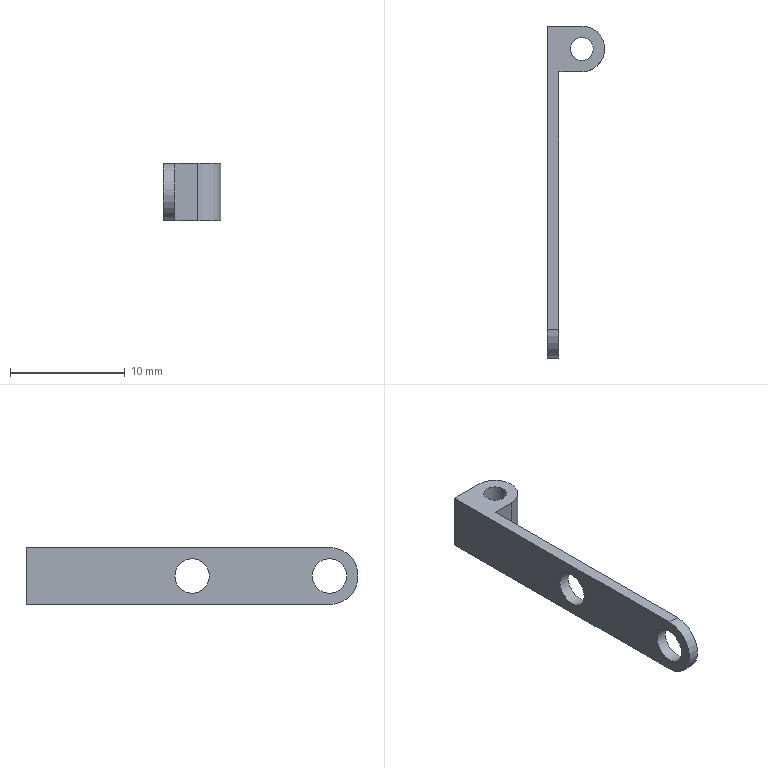Part | STEP file | 1-63.2 | 1 solid | 11 faces | box 5 x 29 x 5 mm | volume 183.888 mm3 | plane 6 | cylinder 5 | commonest cylinder face diameters 3 x2 2 x1 4 x1 5 x1
STEP:
#1=CARTESIAN_POINT('',(0.,0.,0.));
#2=DIRECTION('',(0.,0.,1.));
#3=DIRECTION('',(1.,0.,0.));
#4=AXIS2_PLACEMENT_3D('',#1,#2,#3);
#5=CARTESIAN_POINT('',(0.,0.,2.5));
#6=VERTEX_POINT('',#5);
#7=CARTESIAN_POINT('',(0.,0.,-2.5));
#8=VERTEX_POINT('',#7);
#9=CARTESIAN_POINT('',(0.,0.,0.));
#10=DIRECTION('',(1.,0.,0.));
#11=DIRECTION('',(0.,0.,1.));
#12=AXIS2_PLACEMENT_3D('',#9,#10,#11);
#13=CIRCLE('',#12,2.5);
#14=CARTESIAN_POINT('',(0.,0.,0.));
#15=DIRECTION('',(1.,0.,0.));
#16=DIRECTION('',(0.,0.,1.));
#17=AXIS2_PLACEMENT_3D('',#14,#15,#16);
#18=CYLINDRICAL_SURFACE('',#17,2.5);
#19=CARTESIAN_POINT('',(0.,0.));
#20=DIRECTION('',(1.,0.));
#21=VECTOR('',#20,1.);
#22=LINE('',#19,#21);
#23=(GEOMETRIC_REPRESENTATION_CONTEXT(2)PARAMETRIC_REPRESENTATION_CONTEXT()REPRESENTATION_CONTEXT('',''));
#24=DEFINITIONAL_REPRESENTATION('',(#22),#23);
#25=PCURVE('',#18,#24);
#26=CARTESIAN_POINT('',(0.,14.25,14.25));
#27=DIRECTION('',(1.,0.,0.));
#28=DIRECTION('',(0.,1.,0.));
#29=AXIS2_PLACEMENT_3D('',#26,#27,#28);
#30=PLANE('',#29);
#31=CARTESIAN_POINT('',(-14.25,-14.25));
#32=DIRECTION('',(0.,1.));
#33=AXIS2_PLACEMENT_2D('',#31,#32);
#34=CIRCLE('',#33,2.5);
#35=(GEOMETRIC_REPRESENTATION_CONTEXT(2)PARAMETRIC_REPRESENTATION_CONTEXT()REPRESENTATION_CONTEXT('',''));
#36=DEFINITIONAL_REPRESENTATION('',(#34),#35);
#37=PCURVE('',#30,#36);
#38=SURFACE_CURVE('',#13,(#25,#37),.PCURVE_S1.);
#39=EDGE_CURVE('',#6,#8,#38,.T.);
#40=ORIENTED_EDGE('',*,*,#39,.T.);
#41=CARTESIAN_POINT('',(1.,0.,-2.5));
#42=VERTEX_POINT('',#41);
#43=CARTESIAN_POINT('',(0.,0.,-2.5));
#44=DIRECTION('',(1.,0.,0.));
#45=VECTOR('',#44,1.);
#46=LINE('',#43,#45);
#47=CARTESIAN_POINT('',(3.142,0.));
#48=DIRECTION('',(0.,1.));
#49=VECTOR('',#48,1.);
#50=LINE('',#47,#49);
#51=(GEOMETRIC_REPRESENTATION_CONTEXT(2)PARAMETRIC_REPRESENTATION_CONTEXT()REPRESENTATION_CONTEXT('',''));
#52=DEFINITIONAL_REPRESENTATION('',(#50),#51);
#53=PCURVE('',#18,#52);
#54=CARTESIAN_POINT('',(2.6,15.5,-2.5));
#55=DIRECTION('',(0.,0.,-1.));
#56=DIRECTION('',(0.,1.,0.));
#57=AXIS2_PLACEMENT_3D('',#54,#55,#56);
#58=PLANE('',#57);
#59=CARTESIAN_POINT('',(-15.5,-2.6));
#60=DIRECTION('',(0.,1.));
#61=VECTOR('',#60,1.);
#62=LINE('',#59,#61);
#63=(GEOMETRIC_REPRESENTATION_CONTEXT(2)PARAMETRIC_REPRESENTATION_CONTEXT()REPRESENTATION_CONTEXT('',''));
#64=DEFINITIONAL_REPRESENTATION('',(#62),#63);
#65=PCURVE('',#58,#64);
#66=SURFACE_CURVE('',#46,(#53,#65),.PCURVE_S1.);
#67=EDGE_CURVE('',#8,#42,#66,.T.);
#68=ORIENTED_EDGE('',*,*,#67,.T.);
#69=CARTESIAN_POINT('',(1.,0.,2.5));
#70=VERTEX_POINT('',#69);
#71=CARTESIAN_POINT('',(1.,0.,0.));
#72=DIRECTION('',(1.,0.,0.));
#73=DIRECTION('',(0.,0.,1.));
#74=AXIS2_PLACEMENT_3D('',#71,#72,#73);
#75=CIRCLE('',#74,2.5);
#76=CARTESIAN_POINT('',(0.,1.));
#77=DIRECTION('',(1.,0.));
#78=VECTOR('',#77,1.);
#79=LINE('',#76,#78);
#80=(GEOMETRIC_REPRESENTATION_CONTEXT(2)PARAMETRIC_REPRESENTATION_CONTEXT()REPRESENTATION_CONTEXT('',''));
#81=DEFINITIONAL_REPRESENTATION('',(#79),#80);
#82=PCURVE('',#18,#81);
#83=CARTESIAN_POINT('',(1.,14.25,0.));
#84=DIRECTION('',(1.,0.,0.));
#85=DIRECTION('',(0.,1.,0.));
#86=AXIS2_PLACEMENT_3D('',#83,#84,#85);
#87=PLANE('',#86);
#88=CARTESIAN_POINT('',(-14.25,0.));
#89=DIRECTION('',(0.,1.));
#90=AXIS2_PLACEMENT_2D('',#88,#89);
#91=CIRCLE('',#90,2.5);
#92=(GEOMETRIC_REPRESENTATION_CONTEXT(2)PARAMETRIC_REPRESENTATION_CONTEXT()REPRESENTATION_CONTEXT('',''));
#93=DEFINITIONAL_REPRESENTATION('',(#91),#92);
#94=PCURVE('',#87,#93);
#95=SURFACE_CURVE('',#75,(#82,#94),.PCURVE_S1.);
#96=EDGE_CURVE('',#70,#42,#95,.T.);
#97=ORIENTED_EDGE('',*,*,#96,.F.);
#98=CARTESIAN_POINT('',(0.,0.,2.5));
#99=DIRECTION('',(1.,0.,0.));
#100=VECTOR('',#99,1.);
#101=LINE('',#98,#100);
#102=CARTESIAN_POINT('',(0.,0.));
#103=DIRECTION('',(0.,1.));
#104=VECTOR('',#103,1.);
#105=LINE('',#102,#104);
#106=(GEOMETRIC_REPRESENTATION_CONTEXT(2)PARAMETRIC_REPRESENTATION_CONTEXT()REPRESENTATION_CONTEXT('',''));
#107=DEFINITIONAL_REPRESENTATION('',(#105),#106);
#108=PCURVE('',#18,#107);
#109=CARTESIAN_POINT('',(2.6,15.5,2.5));
#110=DIRECTION('',(0.,0.,1.));
#111=DIRECTION('',(0.,-1.,0.));
#112=AXIS2_PLACEMENT_3D('',#109,#110,#111);
#113=PLANE('',#112);
#114=CARTESIAN_POINT('',(15.5,-2.6));
#115=DIRECTION('',(0.,1.));
#116=VECTOR('',#115,1.);
#117=LINE('',#114,#116);
#118=(GEOMETRIC_REPRESENTATION_CONTEXT(2)PARAMETRIC_REPRESENTATION_CONTEXT()REPRESENTATION_CONTEXT('',''));
#119=DEFINITIONAL_REPRESENTATION('',(#117),#118);
#120=PCURVE('',#113,#119);
#121=SURFACE_CURVE('',#101,(#108,#120),.PCURVE_S1.);
#122=EDGE_CURVE('',#6,#70,#121,.T.);
#123=ORIENTED_EDGE('',*,*,#122,.F.);
#124=EDGE_LOOP('',(#40,#68,#97,#123));
#125=FACE_BOUND('',#124,.T.);
#126=ADVANCED_FACE('',(#125),#18,.T.);
#127=CARTESIAN_POINT('',(0.,1.5,0.));
#128=VERTEX_POINT('',#127);
#129=CARTESIAN_POINT('',(1.,1.5,0.));
#130=VERTEX_POINT('',#129);
#131=CARTESIAN_POINT('',(0.,1.5,0.));
#132=DIRECTION('',(1.,0.,0.));
#133=VECTOR('',#132,1.);
#134=LINE('',#131,#133);
#135=CARTESIAN_POINT('',(0.,0.,0.));
#136=DIRECTION('',(1.,0.,0.));
#137=DIRECTION('',(0.,1.,0.));
#138=AXIS2_PLACEMENT_3D('',#135,#136,#137);
#139=CYLINDRICAL_SURFACE('',#138,1.5);
#140=CARTESIAN_POINT('',(6.283,0.));
#141=DIRECTION('',(0.,1.));
#142=VECTOR('',#141,1.);
#143=LINE('',#140,#142);
#144=(GEOMETRIC_REPRESENTATION_CONTEXT(2)PARAMETRIC_REPRESENTATION_CONTEXT()REPRESENTATION_CONTEXT('',''));
#145=DEFINITIONAL_REPRESENTATION('',(#143),#144);
#146=PCURVE('',#139,#145);
#147=CARTESIAN_POINT('',(0.,0.));
#148=DIRECTION('',(0.,1.));
#149=VECTOR('',#148,1.);
#150=LINE('',#147,#149);
#151=(GEOMETRIC_REPRESENTATION_CONTEXT(2)PARAMETRIC_REPRESENTATION_CONTEXT()REPRESENTATION_CONTEXT('',''));
#152=DEFINITIONAL_REPRESENTATION('',(#150),#151);
#153=PCURVE('',#139,#152);
#154=SEAM_CURVE('',#134,(#146,#153),.PCURVE_S1.);
#155=EDGE_CURVE('',#128,#130,#154,.T.);
#156=ORIENTED_EDGE('',*,*,#155,.T.);
#157=CARTESIAN_POINT('',(1.,0.,0.));
#158=DIRECTION('',(-1.,0.,0.));
#159=DIRECTION('',(0.,1.,0.));
#160=AXIS2_PLACEMENT_3D('',#157,#158,#159);
#161=CIRCLE('',#160,1.5);
#162=CARTESIAN_POINT('',(6.283,1.));
#163=DIRECTION('',(-1.,0.));
#164=VECTOR('',#163,1.);
#165=LINE('',#162,#164);
#166=(GEOMETRIC_REPRESENTATION_CONTEXT(2)PARAMETRIC_REPRESENTATION_CONTEXT()REPRESENTATION_CONTEXT('',''));
#167=DEFINITIONAL_REPRESENTATION('',(#165),#166);
#168=PCURVE('',#139,#167);
#169=CARTESIAN_POINT('',(-12.75,0.));
#170=CARTESIAN_POINT('',(-12.75,-2.598));
#171=CARTESIAN_POINT('',(-15.,-1.299));
#172=CARTESIAN_POINT('',(-17.25,0.));
#173=CARTESIAN_POINT('',(-15.,1.299));
#174=CARTESIAN_POINT('',(-12.75,2.598));
#175=CARTESIAN_POINT('',(-12.75,0.));
#176=(BOUNDED_CURVE()B_SPLINE_CURVE(2,(#169,#170,#171,#172,#173,#174,#175),.UNSPECIFIED.,.T.,.F.)B_SPLINE_CURVE_WITH_KNOTS((1,2,2,2,2,1),(-2.094,0.,2.094,4.189,6.283,8.378),.UNSPECIFIED.)CURVE()GEOMETRIC_REPRESENTATION_ITEM()RATIONAL_B_SPLINE_CURVE((1.,0.5,1.,0.5,1.,0.5,1.))REPRESENTATION_ITEM(''));
#177=(GEOMETRIC_REPRESENTATION_CONTEXT(2)PARAMETRIC_REPRESENTATION_CONTEXT()REPRESENTATION_CONTEXT('',''));
#178=DEFINITIONAL_REPRESENTATION('',(#176),#177);
#179=PCURVE('',#87,#178);
#180=SURFACE_CURVE('',#161,(#168,#179),.PCURVE_S1.);
#181=EDGE_CURVE('',#130,#130,#180,.T.);
#182=ORIENTED_EDGE('',*,*,#181,.T.);
#183=ORIENTED_EDGE('',*,*,#155,.F.);
#184=CARTESIAN_POINT('',(0.,0.,0.));
#185=DIRECTION('',(-1.,0.,0.));
#186=DIRECTION('',(0.,1.,0.));
#187=AXIS2_PLACEMENT_3D('',#184,#185,#186);
#188=CIRCLE('',#187,1.5);
#189=CARTESIAN_POINT('',(6.283,0.));
#190=DIRECTION('',(-1.,0.));
#191=VECTOR('',#190,1.);
#192=LINE('',#189,#191);
#193=(GEOMETRIC_REPRESENTATION_CONTEXT(2)PARAMETRIC_REPRESENTATION_CONTEXT()REPRESENTATION_CONTEXT('',''));
#194=DEFINITIONAL_REPRESENTATION('',(#192),#193);
#195=PCURVE('',#139,#194);
#196=CARTESIAN_POINT('',(-12.75,-14.25));
#197=CARTESIAN_POINT('',(-12.75,-16.848));
#198=CARTESIAN_POINT('',(-15.,-15.549));
#199=CARTESIAN_POINT('',(-17.25,-14.25));
#200=CARTESIAN_POINT('',(-15.,-12.951));
#201=CARTESIAN_POINT('',(-12.75,-11.652));
#202=CARTESIAN_POINT('',(-12.75,-14.25));
#203=(BOUNDED_CURVE()B_SPLINE_CURVE(2,(#196,#197,#198,#199,#200,#201,#202),.UNSPECIFIED.,.T.,.F.)B_SPLINE_CURVE_WITH_KNOTS((1,2,2,2,2,1),(-2.094,0.,2.094,4.189,6.283,8.378),.UNSPECIFIED.)CURVE()GEOMETRIC_REPRESENTATION_ITEM()RATIONAL_B_SPLINE_CURVE((1.,0.5,1.,0.5,1.,0.5,1.))REPRESENTATION_ITEM(''));
#204=(GEOMETRIC_REPRESENTATION_CONTEXT(2)PARAMETRIC_REPRESENTATION_CONTEXT()REPRESENTATION_CONTEXT('',''));
#205=DEFINITIONAL_REPRESENTATION('',(#203),#204);
#206=PCURVE('',#30,#205);
#207=SURFACE_CURVE('',#188,(#195,#206),.PCURVE_S1.);
#208=EDGE_CURVE('',#128,#128,#207,.T.);
#209=ORIENTED_EDGE('',*,*,#208,.F.);
#210=EDGE_LOOP('',(#156,#182,#183,#209));
#211=FACE_BOUND('',#210,.F.);
#212=ADVANCED_FACE('',(#211),#139,.F.);
#213=CARTESIAN_POINT('',(0.,13.5,0.));
#214=VERTEX_POINT('',#213);
#215=CARTESIAN_POINT('',(1.,13.5,0.));
#216=VERTEX_POINT('',#215);
#217=CARTESIAN_POINT('',(0.,13.5,0.));
#218=DIRECTION('',(1.,0.,0.));
#219=VECTOR('',#218,1.);
#220=LINE('',#217,#219);
#221=CARTESIAN_POINT('',(0.,12.,0.));
#222=DIRECTION('',(1.,0.,0.));
#223=DIRECTION('',(0.,1.,0.));
#224=AXIS2_PLACEMENT_3D('',#221,#222,#223);
#225=CYLINDRICAL_SURFACE('',#224,1.5);
#226=CARTESIAN_POINT('',(6.283,0.));
#227=DIRECTION('',(0.,1.));
#228=VECTOR('',#227,1.);
#229=LINE('',#226,#228);
#230=(GEOMETRIC_REPRESENTATION_CONTEXT(2)PARAMETRIC_REPRESENTATION_CONTEXT()REPRESENTATION_CONTEXT('',''));
#231=DEFINITIONAL_REPRESENTATION('',(#229),#230);
#232=PCURVE('',#225,#231);
#233=CARTESIAN_POINT('',(0.,0.));
#234=DIRECTION('',(0.,1.));
#235=VECTOR('',#234,1.);
#236=LINE('',#233,#235);
#237=(GEOMETRIC_REPRESENTATION_CONTEXT(2)PARAMETRIC_REPRESENTATION_CONTEXT()REPRESENTATION_CONTEXT('',''));
#238=DEFINITIONAL_REPRESENTATION('',(#236),#237);
#239=PCURVE('',#225,#238);
#240=SEAM_CURVE('',#220,(#232,#239),.PCURVE_S1.);
#241=EDGE_CURVE('',#214,#216,#240,.T.);
#242=ORIENTED_EDGE('',*,*,#241,.T.);
#243=CARTESIAN_POINT('',(1.,12.,0.));
#244=DIRECTION('',(-1.,0.,0.));
#245=DIRECTION('',(0.,1.,0.));
#246=AXIS2_PLACEMENT_3D('',#243,#244,#245);
#247=CIRCLE('',#246,1.5);
#248=CARTESIAN_POINT('',(6.283,1.));
#249=DIRECTION('',(-1.,0.));
#250=VECTOR('',#249,1.);
#251=LINE('',#248,#250);
#252=(GEOMETRIC_REPRESENTATION_CONTEXT(2)PARAMETRIC_REPRESENTATION_CONTEXT()REPRESENTATION_CONTEXT('',''));
#253=DEFINITIONAL_REPRESENTATION('',(#251),#252);
#254=PCURVE('',#225,#253);
#255=CARTESIAN_POINT('',(-0.75,0.));
#256=CARTESIAN_POINT('',(-0.75,-2.598));
#257=CARTESIAN_POINT('',(-3.,-1.299));
#258=CARTESIAN_POINT('',(-5.25,0.));
#259=CARTESIAN_POINT('',(-3.,1.299));
#260=CARTESIAN_POINT('',(-0.75,2.598));
#261=CARTESIAN_POINT('',(-0.75,0.));
#262=(BOUNDED_CURVE()B_SPLINE_CURVE(2,(#255,#256,#257,#258,#259,#260,#261),.UNSPECIFIED.,.T.,.F.)B_SPLINE_CURVE_WITH_KNOTS((1,2,2,2,2,1),(-2.094,0.,2.094,4.189,6.283,8.378),.UNSPECIFIED.)CURVE()GEOMETRIC_REPRESENTATION_ITEM()RATIONAL_B_SPLINE_CURVE((1.,0.5,1.,0.5,1.,0.5,1.))REPRESENTATION_ITEM(''));
#263=(GEOMETRIC_REPRESENTATION_CONTEXT(2)PARAMETRIC_REPRESENTATION_CONTEXT()REPRESENTATION_CONTEXT('',''));
#264=DEFINITIONAL_REPRESENTATION('',(#262),#263);
#265=PCURVE('',#87,#264);
#266=SURFACE_CURVE('',#247,(#254,#265),.PCURVE_S1.);
#267=EDGE_CURVE('',#216,#216,#266,.T.);
#268=ORIENTED_EDGE('',*,*,#267,.T.);
#269=ORIENTED_EDGE('',*,*,#241,.F.);
#270=CARTESIAN_POINT('',(0.,12.,0.));
#271=DIRECTION('',(-1.,0.,0.));
#272=DIRECTION('',(0.,1.,0.));
#273=AXIS2_PLACEMENT_3D('',#270,#271,#272);
#274=CIRCLE('',#273,1.5);
#275=CARTESIAN_POINT('',(6.283,0.));
#276=DIRECTION('',(-1.,0.));
#277=VECTOR('',#276,1.);
#278=LINE('',#275,#277);
#279=(GEOMETRIC_REPRESENTATION_CONTEXT(2)PARAMETRIC_REPRESENTATION_CONTEXT()REPRESENTATION_CONTEXT('',''));
#280=DEFINITIONAL_REPRESENTATION('',(#278),#279);
#281=PCURVE('',#225,#280);
#282=CARTESIAN_POINT('',(-0.75,-14.25));
#283=CARTESIAN_POINT('',(-0.75,-16.848));
#284=CARTESIAN_POINT('',(-3.,-15.549));
#285=CARTESIAN_POINT('',(-5.25,-14.25));
#286=CARTESIAN_POINT('',(-3.,-12.951));
#287=CARTESIAN_POINT('',(-0.75,-11.652));
#288=CARTESIAN_POINT('',(-0.75,-14.25));
#289=(BOUNDED_CURVE()B_SPLINE_CURVE(2,(#282,#283,#284,#285,#286,#287,#288),.UNSPECIFIED.,.T.,.F.)B_SPLINE_CURVE_WITH_KNOTS((1,2,2,2,2,1),(-2.094,0.,2.094,4.189,6.283,8.378),.UNSPECIFIED.)CURVE()GEOMETRIC_REPRESENTATION_ITEM()RATIONAL_B_SPLINE_CURVE((1.,0.5,1.,0.5,1.,0.5,1.))REPRESENTATION_ITEM(''));
#290=(GEOMETRIC_REPRESENTATION_CONTEXT(2)PARAMETRIC_REPRESENTATION_CONTEXT()REPRESENTATION_CONTEXT('',''));
#291=DEFINITIONAL_REPRESENTATION('',(#289),#290);
#292=PCURVE('',#30,#291);
#293=SURFACE_CURVE('',#274,(#281,#292),.PCURVE_S1.);
#294=EDGE_CURVE('',#214,#214,#293,.T.);
#295=ORIENTED_EDGE('',*,*,#294,.F.);
#296=EDGE_LOOP('',(#242,#268,#269,#295));
#297=FACE_BOUND('',#296,.F.);
#298=ADVANCED_FACE('',(#297),#225,.F.);
#299=ORIENTED_EDGE('',*,*,#96,.T.);
#300=CARTESIAN_POINT('',(1.,22.5,-2.5));
#301=VERTEX_POINT('',#300);
#302=CARTESIAN_POINT('',(1.,0.,-2.5));
#303=DIRECTION('',(0.,1.,0.));
#304=VECTOR('',#303,1.);
#305=LINE('',#302,#304);
#306=CARTESIAN_POINT('',(-14.25,-2.5));
#307=DIRECTION('',(1.,0.));
#308=VECTOR('',#307,1.);
#309=LINE('',#306,#308);
#310=(GEOMETRIC_REPRESENTATION_CONTEXT(2)PARAMETRIC_REPRESENTATION_CONTEXT()REPRESENTATION_CONTEXT('',''));
#311=DEFINITIONAL_REPRESENTATION('',(#309),#310);
#312=PCURVE('',#87,#311);
#313=CARTESIAN_POINT('',(-15.5,-1.6));
#314=DIRECTION('',(1.,0.));
#315=VECTOR('',#314,1.);
#316=LINE('',#313,#315);
#317=(GEOMETRIC_REPRESENTATION_CONTEXT(2)PARAMETRIC_REPRESENTATION_CONTEXT()REPRESENTATION_CONTEXT('',''));
#318=DEFINITIONAL_REPRESENTATION('',(#316),#317);
#319=PCURVE('',#58,#318);
#320=SURFACE_CURVE('',#305,(#312,#319),.PCURVE_S1.);
#321=EDGE_CURVE('',#42,#301,#320,.T.);
#322=ORIENTED_EDGE('',*,*,#321,.T.);
#323=CARTESIAN_POINT('',(1.,22.5,2.5));
#324=VERTEX_POINT('',#323);
#325=CARTESIAN_POINT('',(1.,22.5,-2.5));
#326=DIRECTION('',(0.,0.,1.));
#327=VECTOR('',#326,1.);
#328=LINE('',#325,#327);
#329=CARTESIAN_POINT('',(8.25,-2.5));
#330=DIRECTION('',(0.,1.));
#331=VECTOR('',#330,1.);
#332=LINE('',#329,#331);
#333=(GEOMETRIC_REPRESENTATION_CONTEXT(2)PARAMETRIC_REPRESENTATION_CONTEXT()REPRESENTATION_CONTEXT('',''));
#334=DEFINITIONAL_REPRESENTATION('',(#332),#333);
#335=PCURVE('',#87,#334);
#336=CARTESIAN_POINT('',(2.,22.5,0.));
#337=DIRECTION('',(0.,-1.,0.));
#338=DIRECTION('',(1.,0.,0.));
#339=AXIS2_PLACEMENT_3D('',#336,#337,#338);
#340=PLANE('',#339);
#341=CARTESIAN_POINT('',(-1.,-2.5));
#342=DIRECTION('',(0.,1.));
#343=VECTOR('',#342,1.);
#344=LINE('',#341,#343);
#345=(GEOMETRIC_REPRESENTATION_CONTEXT(2)PARAMETRIC_REPRESENTATION_CONTEXT()REPRESENTATION_CONTEXT('',''));
#346=DEFINITIONAL_REPRESENTATION('',(#344),#345);
#347=PCURVE('',#340,#346);
#348=SURFACE_CURVE('',#328,(#335,#347),.PCURVE_S1.);
#349=EDGE_CURVE('',#301,#324,#348,.T.);
#350=ORIENTED_EDGE('',*,*,#349,.T.);
#351=CARTESIAN_POINT('',(1.,22.5,2.5));
#352=DIRECTION('',(0.,-1.,0.));
#353=VECTOR('',#352,1.);
#354=LINE('',#351,#353);
#355=CARTESIAN_POINT('',(8.25,2.5));
#356=DIRECTION('',(-1.,0.));
#357=VECTOR('',#356,1.);
#358=LINE('',#355,#357);
#359=(GEOMETRIC_REPRESENTATION_CONTEXT(2)PARAMETRIC_REPRESENTATION_CONTEXT()REPRESENTATION_CONTEXT('',''));
#360=DEFINITIONAL_REPRESENTATION('',(#358),#359);
#361=PCURVE('',#87,#360);
#362=CARTESIAN_POINT('',(-7.,-1.6));
#363=DIRECTION('',(1.,0.));
#364=VECTOR('',#363,1.);
#365=LINE('',#362,#364);
#366=(GEOMETRIC_REPRESENTATION_CONTEXT(2)PARAMETRIC_REPRESENTATION_CONTEXT()REPRESENTATION_CONTEXT('',''));
#367=DEFINITIONAL_REPRESENTATION('',(#365),#366);
#368=PCURVE('',#113,#367);
#369=SURFACE_CURVE('',#354,(#361,#368),.PCURVE_S1.);
#370=EDGE_CURVE('',#324,#70,#369,.T.);
#371=ORIENTED_EDGE('',*,*,#370,.T.);
#372=EDGE_LOOP('',(#299,#322,#350,#371));
#373=FACE_BOUND('',#372,.T.);
#374=ORIENTED_EDGE('',*,*,#181,.T.);
#375=EDGE_LOOP('',(#374));
#376=FACE_BOUND('',#375,.T.);
#377=ORIENTED_EDGE('',*,*,#267,.T.);
#378=EDGE_LOOP('',(#377));
#379=FACE_BOUND('',#378,.T.);
#380=ADVANCED_FACE('',(#373,#376,#379),#87,.T.);
#381=CARTESIAN_POINT('',(3.,22.5,-2.5));
#382=VERTEX_POINT('',#381);
#383=CARTESIAN_POINT('',(1.,22.5,-2.5));
#384=DIRECTION('',(1.,0.,0.));
#385=VECTOR('',#384,1.);
#386=LINE('',#383,#385);
#387=CARTESIAN_POINT('',(-1.,-2.5));
#388=DIRECTION('',(1.,0.));
#389=VECTOR('',#388,1.);
#390=LINE('',#387,#389);
#391=(GEOMETRIC_REPRESENTATION_CONTEXT(2)PARAMETRIC_REPRESENTATION_CONTEXT()REPRESENTATION_CONTEXT('',''));
#392=DEFINITIONAL_REPRESENTATION('',(#390),#391);
#393=PCURVE('',#340,#392);
#394=CARTESIAN_POINT('',(7.,-1.6));
#395=DIRECTION('',(0.,1.));
#396=VECTOR('',#395,1.);
#397=LINE('',#394,#396);
#398=(GEOMETRIC_REPRESENTATION_CONTEXT(2)PARAMETRIC_REPRESENTATION_CONTEXT()REPRESENTATION_CONTEXT('',''));
#399=DEFINITIONAL_REPRESENTATION('',(#397),#398);
#400=PCURVE('',#58,#399);
#401=SURFACE_CURVE('',#386,(#393,#400),.PCURVE_S1.);
#402=EDGE_CURVE('',#301,#382,#401,.T.);
#403=ORIENTED_EDGE('',*,*,#402,.T.);
#404=CARTESIAN_POINT('',(3.,22.5,2.5));
#405=VERTEX_POINT('',#404);
#406=CARTESIAN_POINT('',(3.,22.5,-2.5));
#407=DIRECTION('',(0.,0.,1.));
#408=VECTOR('',#407,1.);
#409=LINE('',#406,#408);
#410=CARTESIAN_POINT('',(1.,-2.5));
#411=DIRECTION('',(0.,1.));
#412=VECTOR('',#411,1.);
#413=LINE('',#410,#412);
#414=(GEOMETRIC_REPRESENTATION_CONTEXT(2)PARAMETRIC_REPRESENTATION_CONTEXT()REPRESENTATION_CONTEXT('',''));
#415=DEFINITIONAL_REPRESENTATION('',(#413),#414);
#416=PCURVE('',#340,#415);
#417=CARTESIAN_POINT('',(3.,24.5,-2.5));
#418=DIRECTION('',(0.,0.,1.));
#419=DIRECTION('',(0.,-1.,0.));
#420=AXIS2_PLACEMENT_3D('',#417,#418,#419);
#421=CYLINDRICAL_SURFACE('',#420,2.);
#422=CARTESIAN_POINT('',(0.,0.));
#423=DIRECTION('',(0.,1.));
#424=VECTOR('',#423,1.);
#425=LINE('',#422,#424);
#426=(GEOMETRIC_REPRESENTATION_CONTEXT(2)PARAMETRIC_REPRESENTATION_CONTEXT()REPRESENTATION_CONTEXT('',''));
#427=DEFINITIONAL_REPRESENTATION('',(#425),#426);
#428=PCURVE('',#421,#427);
#429=SURFACE_CURVE('',#409,(#416,#428),.PCURVE_S1.);
#430=EDGE_CURVE('',#382,#405,#429,.T.);
#431=ORIENTED_EDGE('',*,*,#430,.T.);
#432=CARTESIAN_POINT('',(1.,22.5,2.5));
#433=DIRECTION('',(1.,0.,0.));
#434=VECTOR('',#433,1.);
#435=LINE('',#432,#434);
#436=CARTESIAN_POINT('',(-1.,2.5));
#437=DIRECTION('',(1.,0.));
#438=VECTOR('',#437,1.);
#439=LINE('',#436,#438);
#440=(GEOMETRIC_REPRESENTATION_CONTEXT(2)PARAMETRIC_REPRESENTATION_CONTEXT()REPRESENTATION_CONTEXT('',''));
#441=DEFINITIONAL_REPRESENTATION('',(#439),#440);
#442=PCURVE('',#340,#441);
#443=CARTESIAN_POINT('',(-7.,-1.6));
#444=DIRECTION('',(0.,1.));
#445=VECTOR('',#444,1.);
#446=LINE('',#443,#445);
#447=(GEOMETRIC_REPRESENTATION_CONTEXT(2)PARAMETRIC_REPRESENTATION_CONTEXT()REPRESENTATION_CONTEXT('',''));
#448=DEFINITIONAL_REPRESENTATION('',(#446),#447);
#449=PCURVE('',#113,#448);
#450=SURFACE_CURVE('',#435,(#442,#449),.PCURVE_S1.);
#451=EDGE_CURVE('',#324,#405,#450,.T.);
#452=ORIENTED_EDGE('',*,*,#451,.F.);
#453=ORIENTED_EDGE('',*,*,#349,.F.);
#454=EDGE_LOOP('',(#403,#431,#452,#453));
#455=FACE_BOUND('',#454,.T.);
#456=ADVANCED_FACE('',(#455),#340,.T.);
#457=CARTESIAN_POINT('',(3.,26.5,-2.5));
#458=VERTEX_POINT('',#457);
#459=CARTESIAN_POINT('',(3.,26.5,2.5));
#460=VERTEX_POINT('',#459);
#461=CARTESIAN_POINT('',(3.,26.5,-2.5));
#462=DIRECTION('',(0.,0.,1.));
#463=VECTOR('',#462,1.);
#464=LINE('',#461,#463);
#465=CARTESIAN_POINT('',(0.5,26.5,0.));
#466=DIRECTION('',(0.,1.,0.));
#467=DIRECTION('',(-1.,0.,0.));
#468=AXIS2_PLACEMENT_3D('',#465,#466,#467);
#469=PLANE('',#468);
#470=CARTESIAN_POINT('',(-2.5,-2.5));
#471=DIRECTION('',(0.,1.));
#472=VECTOR('',#471,1.);
#473=LINE('',#470,#472);
#474=(GEOMETRIC_REPRESENTATION_CONTEXT(2)PARAMETRIC_REPRESENTATION_CONTEXT()REPRESENTATION_CONTEXT('',''));
#475=DEFINITIONAL_REPRESENTATION('',(#473),#474);
#476=PCURVE('',#469,#475);
#477=CARTESIAN_POINT('',(3.142,0.));
#478=DIRECTION('',(0.,1.));
#479=VECTOR('',#478,1.);
#480=LINE('',#477,#479);
#481=(GEOMETRIC_REPRESENTATION_CONTEXT(2)PARAMETRIC_REPRESENTATION_CONTEXT()REPRESENTATION_CONTEXT('',''));
#482=DEFINITIONAL_REPRESENTATION('',(#480),#481);
#483=PCURVE('',#421,#482);
#484=SURFACE_CURVE('',#464,(#476,#483),.PCURVE_S1.);
#485=EDGE_CURVE('',#458,#460,#484,.T.);
#486=ORIENTED_EDGE('',*,*,#485,.F.);
#487=CARTESIAN_POINT('',(0.,26.5,-2.5));
#488=VERTEX_POINT('',#487);
#489=CARTESIAN_POINT('',(3.,26.5,-2.5));
#490=DIRECTION('',(-1.,0.,0.));
#491=VECTOR('',#490,1.);
#492=LINE('',#489,#491);
#493=CARTESIAN_POINT('',(-2.5,-2.5));
#494=DIRECTION('',(1.,0.));
#495=VECTOR('',#494,1.);
#496=LINE('',#493,#495);
#497=(GEOMETRIC_REPRESENTATION_CONTEXT(2)PARAMETRIC_REPRESENTATION_CONTEXT()REPRESENTATION_CONTEXT('',''));
#498=DEFINITIONAL_REPRESENTATION('',(#496),#497);
#499=PCURVE('',#469,#498);
#500=CARTESIAN_POINT('',(11.,0.4));
#501=DIRECTION('',(0.,-1.));
#502=VECTOR('',#501,1.);
#503=LINE('',#500,#502);
#504=(GEOMETRIC_REPRESENTATION_CONTEXT(2)PARAMETRIC_REPRESENTATION_CONTEXT()REPRESENTATION_CONTEXT('',''));
#505=DEFINITIONAL_REPRESENTATION('',(#503),#504);
#506=PCURVE('',#58,#505);
#507=SURFACE_CURVE('',#492,(#499,#506),.PCURVE_S1.);
#508=EDGE_CURVE('',#458,#488,#507,.T.);
#509=ORIENTED_EDGE('',*,*,#508,.T.);
#510=CARTESIAN_POINT('',(0.,26.5,2.5));
#511=VERTEX_POINT('',#510);
#512=CARTESIAN_POINT('',(0.,26.5,-2.5));
#513=DIRECTION('',(0.,0.,1.));
#514=VECTOR('',#513,1.);
#515=LINE('',#512,#514);
#516=CARTESIAN_POINT('',(0.5,-2.5));
#517=DIRECTION('',(0.,1.));
#518=VECTOR('',#517,1.);
#519=LINE('',#516,#518);
#520=(GEOMETRIC_REPRESENTATION_CONTEXT(2)PARAMETRIC_REPRESENTATION_CONTEXT()REPRESENTATION_CONTEXT('',''));
#521=DEFINITIONAL_REPRESENTATION('',(#519),#520);
#522=PCURVE('',#469,#521);
#523=CARTESIAN_POINT('',(12.25,-16.75));
#524=DIRECTION('',(0.,1.));
#525=VECTOR('',#524,1.);
#526=LINE('',#523,#525);
#527=(GEOMETRIC_REPRESENTATION_CONTEXT(2)PARAMETRIC_REPRESENTATION_CONTEXT()REPRESENTATION_CONTEXT('',''));
#528=DEFINITIONAL_REPRESENTATION('',(#526),#527);
#529=PCURVE('',#30,#528);
#530=SURFACE_CURVE('',#515,(#522,#529),.PCURVE_S1.);
#531=EDGE_CURVE('',#488,#511,#530,.T.);
#532=ORIENTED_EDGE('',*,*,#531,.T.);
#533=CARTESIAN_POINT('',(3.,26.5,2.5));
#534=DIRECTION('',(-1.,0.,0.));
#535=VECTOR('',#534,1.);
#536=LINE('',#533,#535);
#537=CARTESIAN_POINT('',(-2.5,2.5));
#538=DIRECTION('',(1.,0.));
#539=VECTOR('',#538,1.);
#540=LINE('',#537,#539);
#541=(GEOMETRIC_REPRESENTATION_CONTEXT(2)PARAMETRIC_REPRESENTATION_CONTEXT()REPRESENTATION_CONTEXT('',''));
#542=DEFINITIONAL_REPRESENTATION('',(#540),#541);
#543=PCURVE('',#469,#542);
#544=CARTESIAN_POINT('',(-11.,0.4));
#545=DIRECTION('',(0.,-1.));
#546=VECTOR('',#545,1.);
#547=LINE('',#544,#546);
#548=(GEOMETRIC_REPRESENTATION_CONTEXT(2)PARAMETRIC_REPRESENTATION_CONTEXT()REPRESENTATION_CONTEXT('',''));
#549=DEFINITIONAL_REPRESENTATION('',(#547),#548);
#550=PCURVE('',#113,#549);
#551=SURFACE_CURVE('',#536,(#543,#550),.PCURVE_S1.);
#552=EDGE_CURVE('',#460,#511,#551,.T.);
#553=ORIENTED_EDGE('',*,*,#552,.F.);
#554=EDGE_LOOP('',(#486,#509,#532,#553));
#555=FACE_BOUND('',#554,.T.);
#556=ADVANCED_FACE('',(#555),#469,.T.);
#557=CARTESIAN_POINT('',(3.,24.5,-2.5));
#558=DIRECTION('',(0.,0.,1.));
#559=DIRECTION('',(0.,-1.,0.));
#560=AXIS2_PLACEMENT_3D('',#557,#558,#559);
#561=CIRCLE('',#560,2.);
#562=CARTESIAN_POINT('',(0.,0.));
#563=DIRECTION('',(1.,0.));
#564=VECTOR('',#563,1.);
#565=LINE('',#562,#564);
#566=(GEOMETRIC_REPRESENTATION_CONTEXT(2)PARAMETRIC_REPRESENTATION_CONTEXT()REPRESENTATION_CONTEXT('',''));
#567=DEFINITIONAL_REPRESENTATION('',(#565),#566);
#568=PCURVE('',#421,#567);
#569=CARTESIAN_POINT('',(7.,0.4));
#570=CARTESIAN_POINT('',(7.,3.864));
#571=CARTESIAN_POINT('',(10.,2.132));
#572=CARTESIAN_POINT('',(13.,0.4));
#573=CARTESIAN_POINT('',(10.,-1.332));
#574=CARTESIAN_POINT('',(7.,-3.064));
#575=CARTESIAN_POINT('',(7.,0.4));
#576=(BOUNDED_CURVE()B_SPLINE_CURVE(2,(#569,#570,#571,#572,#573,#574,#575),.UNSPECIFIED.,.T.,.F.)B_SPLINE_CURVE_WITH_KNOTS((1,2,2,2,2,1),(-2.094,0.,2.094,4.189,6.283,8.378),.UNSPECIFIED.)CURVE()GEOMETRIC_REPRESENTATION_ITEM()RATIONAL_B_SPLINE_CURVE((1.,0.5,1.,0.5,1.,0.5,1.))REPRESENTATION_ITEM(''));
#577=(GEOMETRIC_REPRESENTATION_CONTEXT(2)PARAMETRIC_REPRESENTATION_CONTEXT()REPRESENTATION_CONTEXT('',''));
#578=DEFINITIONAL_REPRESENTATION('',(#576),#577);
#579=PCURVE('',#58,#578);
#580=SURFACE_CURVE('',#561,(#568,#579),.PCURVE_S1.);
#581=EDGE_CURVE('',#382,#458,#580,.T.);
#582=ORIENTED_EDGE('',*,*,#581,.T.);
#583=ORIENTED_EDGE('',*,*,#485,.T.);
#584=CARTESIAN_POINT('',(3.,24.5,2.5));
#585=DIRECTION('',(0.,0.,1.));
#586=DIRECTION('',(0.,-1.,0.));
#587=AXIS2_PLACEMENT_3D('',#584,#585,#586);
#588=CIRCLE('',#587,2.);
#589=CARTESIAN_POINT('',(0.,5.));
#590=DIRECTION('',(1.,0.));
#591=VECTOR('',#590,1.);
#592=LINE('',#589,#591);
#593=(GEOMETRIC_REPRESENTATION_CONTEXT(2)PARAMETRIC_REPRESENTATION_CONTEXT()REPRESENTATION_CONTEXT('',''));
#594=DEFINITIONAL_REPRESENTATION('',(#592),#593);
#595=PCURVE('',#421,#594);
#596=CARTESIAN_POINT('',(-9.,0.4));
#597=DIRECTION('',(1.,0.));
#598=AXIS2_PLACEMENT_2D('',#596,#597);
#599=CIRCLE('',#598,2.);
#600=(GEOMETRIC_REPRESENTATION_CONTEXT(2)PARAMETRIC_REPRESENTATION_CONTEXT()REPRESENTATION_CONTEXT('',''));
#601=DEFINITIONAL_REPRESENTATION('',(#599),#600);
#602=PCURVE('',#113,#601);
#603=SURFACE_CURVE('',#588,(#595,#602),.PCURVE_S1.);
#604=EDGE_CURVE('',#405,#460,#603,.T.);
#605=ORIENTED_EDGE('',*,*,#604,.F.);
#606=ORIENTED_EDGE('',*,*,#430,.F.);
#607=EDGE_LOOP('',(#582,#583,#605,#606));
#608=FACE_BOUND('',#607,.T.);
#609=ADVANCED_FACE('',(#608),#421,.T.);
#610=CARTESIAN_POINT('',(3.,25.5,-2.5));
#611=VERTEX_POINT('',#610);
#612=CARTESIAN_POINT('',(3.,25.5,2.5));
#613=VERTEX_POINT('',#612);
#614=CARTESIAN_POINT('',(3.,25.5,-2.5));
#615=DIRECTION('',(0.,0.,1.));
#616=VECTOR('',#615,1.);
#617=LINE('',#614,#616);
#618=CARTESIAN_POINT('',(3.,24.5,-2.5));
#619=DIRECTION('',(0.,0.,1.));
#620=DIRECTION('',(0.,1.,0.));
#621=AXIS2_PLACEMENT_3D('',#618,#619,#620);
#622=CYLINDRICAL_SURFACE('',#621,1.);
#623=CARTESIAN_POINT('',(6.283,0.));
#624=DIRECTION('',(0.,1.));
#625=VECTOR('',#624,1.);
#626=LINE('',#623,#625);
#627=(GEOMETRIC_REPRESENTATION_CONTEXT(2)PARAMETRIC_REPRESENTATION_CONTEXT()REPRESENTATION_CONTEXT('',''));
#628=DEFINITIONAL_REPRESENTATION('',(#626),#627);
#629=PCURVE('',#622,#628);
#630=CARTESIAN_POINT('',(0.,0.));
#631=DIRECTION('',(0.,1.));
#632=VECTOR('',#631,1.);
#633=LINE('',#630,#632);
#634=(GEOMETRIC_REPRESENTATION_CONTEXT(2)PARAMETRIC_REPRESENTATION_CONTEXT()REPRESENTATION_CONTEXT('',''));
#635=DEFINITIONAL_REPRESENTATION('',(#633),#634);
#636=PCURVE('',#622,#635);
#637=SEAM_CURVE('',#617,(#629,#636),.PCURVE_S1.);
#638=EDGE_CURVE('',#611,#613,#637,.T.);
#639=ORIENTED_EDGE('',*,*,#638,.T.);
#640=CARTESIAN_POINT('',(3.,24.5,2.5));
#641=DIRECTION('',(0.,0.,-1.));
#642=DIRECTION('',(0.,1.,0.));
#643=AXIS2_PLACEMENT_3D('',#640,#641,#642);
#644=CIRCLE('',#643,1.);
#645=CARTESIAN_POINT('',(6.283,5.));
#646=DIRECTION('',(-1.,0.));
#647=VECTOR('',#646,1.);
#648=LINE('',#645,#647);
#649=(GEOMETRIC_REPRESENTATION_CONTEXT(2)PARAMETRIC_REPRESENTATION_CONTEXT()REPRESENTATION_CONTEXT('',''));
#650=DEFINITIONAL_REPRESENTATION('',(#648),#649);
#651=PCURVE('',#622,#650);
#652=CARTESIAN_POINT('',(-10.,0.4));
#653=CARTESIAN_POINT('',(-10.,2.132));
#654=CARTESIAN_POINT('',(-8.5,1.266));
#655=CARTESIAN_POINT('',(-7.,0.4));
#656=CARTESIAN_POINT('',(-8.5,-0.466));
#657=CARTESIAN_POINT('',(-10.,-1.332));
#658=CARTESIAN_POINT('',(-10.,0.4));
#659=(BOUNDED_CURVE()B_SPLINE_CURVE(2,(#652,#653,#654,#655,#656,#657,#658),.UNSPECIFIED.,.T.,.F.)B_SPLINE_CURVE_WITH_KNOTS((1,2,2,2,2,1),(-2.094,0.,2.094,4.189,6.283,8.378),.UNSPECIFIED.)CURVE()GEOMETRIC_REPRESENTATION_ITEM()RATIONAL_B_SPLINE_CURVE((1.,0.5,1.,0.5,1.,0.5,1.))REPRESENTATION_ITEM(''));
#660=(GEOMETRIC_REPRESENTATION_CONTEXT(2)PARAMETRIC_REPRESENTATION_CONTEXT()REPRESENTATION_CONTEXT('',''));
#661=DEFINITIONAL_REPRESENTATION('',(#659),#660);
#662=PCURVE('',#113,#661);
#663=SURFACE_CURVE('',#644,(#651,#662),.PCURVE_S1.);
#664=EDGE_CURVE('',#613,#613,#663,.T.);
#665=ORIENTED_EDGE('',*,*,#664,.T.);
#666=ORIENTED_EDGE('',*,*,#638,.F.);
#667=CARTESIAN_POINT('',(3.,24.5,-2.5));
#668=DIRECTION('',(0.,0.,-1.));
#669=DIRECTION('',(0.,1.,0.));
#670=AXIS2_PLACEMENT_3D('',#667,#668,#669);
#671=CIRCLE('',#670,1.);
#672=CARTESIAN_POINT('',(6.283,0.));
#673=DIRECTION('',(-1.,0.));
#674=VECTOR('',#673,1.);
#675=LINE('',#672,#674);
#676=(GEOMETRIC_REPRESENTATION_CONTEXT(2)PARAMETRIC_REPRESENTATION_CONTEXT()REPRESENTATION_CONTEXT('',''));
#677=DEFINITIONAL_REPRESENTATION('',(#675),#676);
#678=PCURVE('',#622,#677);
#679=CARTESIAN_POINT('',(9.,0.4));
#680=DIRECTION('',(1.,0.));
#681=AXIS2_PLACEMENT_2D('',#679,#680);
#682=CIRCLE('',#681,1.);
#683=(GEOMETRIC_REPRESENTATION_CONTEXT(2)PARAMETRIC_REPRESENTATION_CONTEXT()REPRESENTATION_CONTEXT('',''));
#684=DEFINITIONAL_REPRESENTATION('',(#682),#683);
#685=PCURVE('',#58,#684);
#686=SURFACE_CURVE('',#671,(#678,#685),.PCURVE_S1.);
#687=EDGE_CURVE('',#611,#611,#686,.T.);
#688=ORIENTED_EDGE('',*,*,#687,.F.);
#689=EDGE_LOOP('',(#639,#665,#666,#688));
#690=FACE_BOUND('',#689,.F.);
#691=ADVANCED_FACE('',(#690),#622,.F.);
#692=ORIENTED_EDGE('',*,*,#39,.T.);
#693=CARTESIAN_POINT('',(0.,0.,-2.5));
#694=DIRECTION('',(0.,1.,0.));
#695=VECTOR('',#694,1.);
#696=LINE('',#693,#695);
#697=CARTESIAN_POINT('',(-14.25,-16.75));
#698=DIRECTION('',(1.,0.));
#699=VECTOR('',#698,1.);
#700=LINE('',#697,#699);
#701=(GEOMETRIC_REPRESENTATION_CONTEXT(2)PARAMETRIC_REPRESENTATION_CONTEXT()REPRESENTATION_CONTEXT('',''));
#702=DEFINITIONAL_REPRESENTATION('',(#700),#701);
#703=PCURVE('',#30,#702);
#704=CARTESIAN_POINT('',(-15.5,-2.6));
#705=DIRECTION('',(1.,0.));
#706=VECTOR('',#705,1.);
#707=LINE('',#704,#706);
#708=(GEOMETRIC_REPRESENTATION_CONTEXT(2)PARAMETRIC_REPRESENTATION_CONTEXT()REPRESENTATION_CONTEXT('',''));
#709=DEFINITIONAL_REPRESENTATION('',(#707),#708);
#710=PCURVE('',#58,#709);
#711=SURFACE_CURVE('',#696,(#703,#710),.PCURVE_S1.);
#712=EDGE_CURVE('',#8,#488,#711,.T.);
#713=ORIENTED_EDGE('',*,*,#712,.T.);
#714=ORIENTED_EDGE('',*,*,#531,.T.);
#715=CARTESIAN_POINT('',(0.,26.5,2.5));
#716=DIRECTION('',(0.,-1.,0.));
#717=VECTOR('',#716,1.);
#718=LINE('',#715,#717);
#719=CARTESIAN_POINT('',(12.25,-11.75));
#720=DIRECTION('',(-1.,0.));
#721=VECTOR('',#720,1.);
#722=LINE('',#719,#721);
#723=(GEOMETRIC_REPRESENTATION_CONTEXT(2)PARAMETRIC_REPRESENTATION_CONTEXT()REPRESENTATION_CONTEXT('',''));
#724=DEFINITIONAL_REPRESENTATION('',(#722),#723);
#725=PCURVE('',#30,#724);
#726=CARTESIAN_POINT('',(-11.,-2.6));
#727=DIRECTION('',(1.,0.));
#728=VECTOR('',#727,1.);
#729=LINE('',#726,#728);
#730=(GEOMETRIC_REPRESENTATION_CONTEXT(2)PARAMETRIC_REPRESENTATION_CONTEXT()REPRESENTATION_CONTEXT('',''));
#731=DEFINITIONAL_REPRESENTATION('',(#729),#730);
#732=PCURVE('',#113,#731);
#733=SURFACE_CURVE('',#718,(#725,#732),.PCURVE_S1.);
#734=EDGE_CURVE('',#511,#6,#733,.T.);
#735=ORIENTED_EDGE('',*,*,#734,.T.);
#736=EDGE_LOOP('',(#692,#713,#714,#735));
#737=FACE_BOUND('',#736,.F.);
#738=ORIENTED_EDGE('',*,*,#208,.T.);
#739=EDGE_LOOP('',(#738));
#740=FACE_BOUND('',#739,.F.);
#741=ORIENTED_EDGE('',*,*,#294,.T.);
#742=EDGE_LOOP('',(#741));
#743=FACE_BOUND('',#742,.F.);
#744=ADVANCED_FACE('',(#737,#740,#743),#30,.F.);
#745=ORIENTED_EDGE('',*,*,#321,.F.);
#746=ORIENTED_EDGE('',*,*,#67,.F.);
#747=ORIENTED_EDGE('',*,*,#712,.T.);
#748=ORIENTED_EDGE('',*,*,#508,.F.);
#749=ORIENTED_EDGE('',*,*,#581,.F.);
#750=ORIENTED_EDGE('',*,*,#402,.F.);
#751=EDGE_LOOP('',(#745,#746,#747,#748,#749,#750));
#752=FACE_BOUND('',#751,.T.);
#753=ORIENTED_EDGE('',*,*,#687,.F.);
#754=EDGE_LOOP('',(#753));
#755=FACE_BOUND('',#754,.T.);
#756=ADVANCED_FACE('',(#752,#755),#58,.T.);
#757=ORIENTED_EDGE('',*,*,#122,.T.);
#758=ORIENTED_EDGE('',*,*,#370,.F.);
#759=ORIENTED_EDGE('',*,*,#451,.T.);
#760=ORIENTED_EDGE('',*,*,#604,.T.);
#761=ORIENTED_EDGE('',*,*,#552,.T.);
#762=ORIENTED_EDGE('',*,*,#734,.T.);
#763=EDGE_LOOP('',(#757,#758,#759,#760,#761,#762));
#764=FACE_BOUND('',#763,.T.);
#765=ORIENTED_EDGE('',*,*,#664,.T.);
#766=EDGE_LOOP('',(#765));
#767=FACE_BOUND('',#766,.T.);
#768=ADVANCED_FACE('',(#764,#767),#113,.T.);
#769=CLOSED_SHELL('',(#126,#212,#298,#380,#456,#556,#609,#691,#744,#756,#768));
#770=MANIFOLD_SOLID_BREP('',#769);
#771=(LENGTH_UNIT()NAMED_UNIT(*)SI_UNIT(.MILLI.,.METRE.));
#772=UNCERTAINTY_MEASURE_WITH_UNIT(LENGTH_MEASURE(0.0000001),#771,'','');
#773=(NAMED_UNIT(*)PLANE_ANGLE_UNIT()SI_UNIT($,.RADIAN.));
#774=(NAMED_UNIT(*)SI_UNIT($,.STERADIAN.)SOLID_ANGLE_UNIT());
#775=(GEOMETRIC_REPRESENTATION_CONTEXT(3)GLOBAL_UNCERTAINTY_ASSIGNED_CONTEXT((#772))GLOBAL_UNIT_ASSIGNED_CONTEXT((#771,#773,#774))REPRESENTATION_CONTEXT('',''));
#776=ADVANCED_BREP_SHAPE_REPRESENTATION('',(#4,#770),#775);